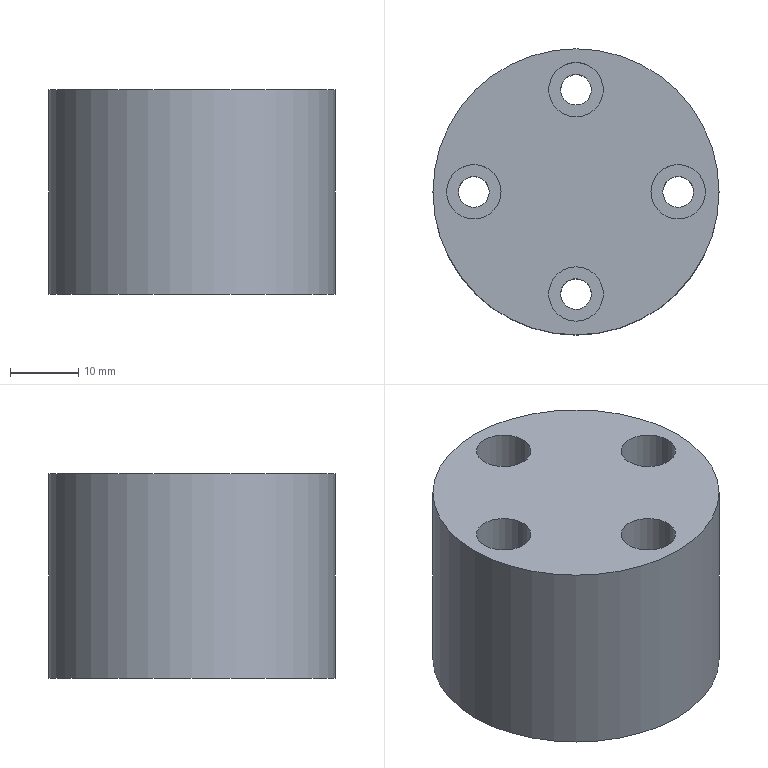Part | NX | 1 solid | 15 faces | box 42 x 42 x 30 mm | volume 38830 mm3 | cylinder 9 | plane 6 | commonest cylinder face diameters 4.5 x4 8 x4 42 x1
STEP:
#1=CARTESIAN_POINT('',(0.,-17.25,-30.));
#2=VERTEX_POINT('',#1);
#3=CARTESIAN_POINT('',(0.,-15.,-30.));
#4=DIRECTION('',(0.,0.,1.));
#5=DIRECTION('',(0.,-1.,0.));
#6=AXIS2_PLACEMENT_3D('',#3,#4,#5);
#7=CIRCLE('',#6,2.25);
#8=EDGE_CURVE('',#2,#2,#7,.T.);
#9=ORIENTED_EDGE('',*,*,#8,.F.);
#10=EDGE_LOOP('',(#9));
#11=FACE_BOUND('',#10,.T.);
#12=CARTESIAN_POINT('',(2.25,-15.,-6.));
#13=VERTEX_POINT('',#12);
#14=CARTESIAN_POINT('',(0.,-15.,-6.));
#15=DIRECTION('',(0.,0.,1.));
#16=DIRECTION('',(1.,0.,0.));
#17=AXIS2_PLACEMENT_3D('',#14,#15,#16);
#18=CIRCLE('',#17,2.25);
#19=EDGE_CURVE('',#13,#13,#18,.T.);
#20=ORIENTED_EDGE('',*,*,#19,.T.);
#21=EDGE_LOOP('',(#20));
#22=FACE_BOUND('',#21,.T.);
#23=CARTESIAN_POINT('',(0.,-15.,0.));
#24=DIRECTION('',(0.,0.,-1.));
#25=DIRECTION('',(-1.,0.,0.));
#26=AXIS2_PLACEMENT_3D('',#23,#24,#25);
#27=CYLINDRICAL_SURFACE('',#26,2.25);
#28=ADVANCED_FACE('',(#11,#22),#27,.F.);
#29=CARTESIAN_POINT('',(0.,17.25,-30.));
#30=VERTEX_POINT('',#29);
#31=CARTESIAN_POINT('',(0.,15.,-30.));
#32=DIRECTION('',(0.,0.,1.));
#33=DIRECTION('',(0.,1.,0.));
#34=AXIS2_PLACEMENT_3D('',#31,#32,#33);
#35=CIRCLE('',#34,2.25);
#36=EDGE_CURVE('',#30,#30,#35,.T.);
#37=ORIENTED_EDGE('',*,*,#36,.F.);
#38=EDGE_LOOP('',(#37));
#39=FACE_BOUND('',#38,.T.);
#40=CARTESIAN_POINT('',(2.25,15.,-6.));
#41=VERTEX_POINT('',#40);
#42=CARTESIAN_POINT('',(0.,15.,-6.));
#43=DIRECTION('',(0.,0.,1.));
#44=DIRECTION('',(1.,0.,0.));
#45=AXIS2_PLACEMENT_3D('',#42,#43,#44);
#46=CIRCLE('',#45,2.25);
#47=EDGE_CURVE('',#41,#41,#46,.T.);
#48=ORIENTED_EDGE('',*,*,#47,.T.);
#49=EDGE_LOOP('',(#48));
#50=FACE_BOUND('',#49,.T.);
#51=CARTESIAN_POINT('',(0.,15.,0.));
#52=DIRECTION('',(0.,0.,-1.));
#53=DIRECTION('',(-1.,0.,0.));
#54=AXIS2_PLACEMENT_3D('',#51,#52,#53);
#55=CYLINDRICAL_SURFACE('',#54,2.25);
#56=ADVANCED_FACE('',(#39,#50),#55,.F.);
#57=CARTESIAN_POINT('',(17.25,0.,-30.));
#58=VERTEX_POINT('',#57);
#59=CARTESIAN_POINT('',(15.,0.,-30.));
#60=DIRECTION('',(0.,0.,1.));
#61=DIRECTION('',(1.,0.,0.));
#62=AXIS2_PLACEMENT_3D('',#59,#60,#61);
#63=CIRCLE('',#62,2.25);
#64=EDGE_CURVE('',#58,#58,#63,.T.);
#65=ORIENTED_EDGE('',*,*,#64,.F.);
#66=EDGE_LOOP('',(#65));
#67=FACE_BOUND('',#66,.T.);
#68=CARTESIAN_POINT('',(17.25,0.,-6.));
#69=VERTEX_POINT('',#68);
#70=CARTESIAN_POINT('',(15.,0.,-6.));
#71=DIRECTION('',(0.,0.,1.));
#72=DIRECTION('',(1.,0.,0.));
#73=AXIS2_PLACEMENT_3D('',#70,#71,#72);
#74=CIRCLE('',#73,2.25);
#75=EDGE_CURVE('',#69,#69,#74,.T.);
#76=ORIENTED_EDGE('',*,*,#75,.T.);
#77=EDGE_LOOP('',(#76));
#78=FACE_BOUND('',#77,.T.);
#79=CARTESIAN_POINT('',(15.,0.,0.));
#80=DIRECTION('',(0.,0.,-1.));
#81=DIRECTION('',(-1.,0.,0.));
#82=AXIS2_PLACEMENT_3D('',#79,#80,#81);
#83=CYLINDRICAL_SURFACE('',#82,2.25);
#84=ADVANCED_FACE('',(#67,#78),#83,.F.);
#85=CARTESIAN_POINT('',(0.,19.,0.));
#86=VERTEX_POINT('',#85);
#87=CARTESIAN_POINT('',(0.,15.,0.));
#88=DIRECTION('',(0.,0.,1.));
#89=DIRECTION('',(0.,1.,0.));
#90=AXIS2_PLACEMENT_3D('',#87,#88,#89);
#91=CIRCLE('',#90,4.);
#92=EDGE_CURVE('',#86,#86,#91,.T.);
#93=ORIENTED_EDGE('',*,*,#92,.F.);
#94=EDGE_LOOP('',(#93));
#95=FACE_BOUND('',#94,.T.);
#96=CARTESIAN_POINT('',(21.,0.,0.));
#97=VERTEX_POINT('',#96);
#98=CARTESIAN_POINT('',(0.,0.,0.));
#99=DIRECTION('',(0.,0.,-1.));
#100=DIRECTION('',(1.,0.,0.));
#101=AXIS2_PLACEMENT_3D('',#98,#99,#100);
#102=CIRCLE('',#101,21.);
#103=EDGE_CURVE('',#97,#97,#102,.T.);
#104=ORIENTED_EDGE('',*,*,#103,.F.);
#105=EDGE_LOOP('',(#104));
#106=FACE_BOUND('',#105,.T.);
#107=CARTESIAN_POINT('',(-19.,0.,0.));
#108=VERTEX_POINT('',#107);
#109=CARTESIAN_POINT('',(-15.,0.,0.));
#110=DIRECTION('',(0.,0.,-1.));
#111=DIRECTION('',(-1.,0.,0.));
#112=AXIS2_PLACEMENT_3D('',#109,#110,#111);
#113=CIRCLE('',#112,4.);
#114=EDGE_CURVE('',#108,#108,#113,.T.);
#115=ORIENTED_EDGE('',*,*,#114,.T.);
#116=EDGE_LOOP('',(#115));
#117=FACE_BOUND('',#116,.T.);
#118=CARTESIAN_POINT('',(0.,-19.,0.));
#119=VERTEX_POINT('',#118);
#120=CARTESIAN_POINT('',(0.,-15.,0.));
#121=DIRECTION('',(0.,0.,1.));
#122=DIRECTION('',(0.,-1.,0.));
#123=AXIS2_PLACEMENT_3D('',#120,#121,#122);
#124=CIRCLE('',#123,4.);
#125=EDGE_CURVE('',#119,#119,#124,.T.);
#126=ORIENTED_EDGE('',*,*,#125,.F.);
#127=EDGE_LOOP('',(#126));
#128=FACE_BOUND('',#127,.T.);
#129=CARTESIAN_POINT('',(19.,0.,0.));
#130=VERTEX_POINT('',#129);
#131=CARTESIAN_POINT('',(15.,0.,0.));
#132=DIRECTION('',(0.,0.,1.));
#133=DIRECTION('',(1.,0.,0.));
#134=AXIS2_PLACEMENT_3D('',#131,#132,#133);
#135=CIRCLE('',#134,4.);
#136=EDGE_CURVE('',#130,#130,#135,.T.);
#137=ORIENTED_EDGE('',*,*,#136,.F.);
#138=EDGE_LOOP('',(#137));
#139=FACE_BOUND('',#138,.T.);
#140=CARTESIAN_POINT('',(7.5,0.,0.));
#141=DIRECTION('',(0.,0.,-1.));
#142=DIRECTION('',(-1.,0.,0.));
#143=AXIS2_PLACEMENT_3D('',#140,#141,#142);
#144=PLANE('',#143);
#145=ADVANCED_FACE('',(#95,#106,#117,#128,#139),#144,.F.);
#146=ORIENTED_EDGE('',*,*,#103,.T.);
#147=EDGE_LOOP('',(#146));
#148=FACE_BOUND('',#147,.T.);
#149=CARTESIAN_POINT('',(21.,0.,-30.));
#150=VERTEX_POINT('',#149);
#151=CARTESIAN_POINT('',(0.,0.,-30.));
#152=DIRECTION('',(0.,0.,-1.));
#153=DIRECTION('',(1.,0.,0.));
#154=AXIS2_PLACEMENT_3D('',#151,#152,#153);
#155=CIRCLE('',#154,21.);
#156=EDGE_CURVE('',#150,#150,#155,.T.);
#157=ORIENTED_EDGE('',*,*,#156,.F.);
#158=EDGE_LOOP('',(#157));
#159=FACE_BOUND('',#158,.T.);
#160=CARTESIAN_POINT('',(0.,0.,0.));
#161=DIRECTION('',(0.,0.,-1.));
#162=DIRECTION('',(-1.,0.,0.));
#163=AXIS2_PLACEMENT_3D('',#160,#161,#162);
#164=CYLINDRICAL_SURFACE('',#163,21.);
#165=ADVANCED_FACE('',(#148,#159),#164,.T.);
#166=CARTESIAN_POINT('',(-17.25,0.,-6.));
#167=VERTEX_POINT('',#166);
#168=CARTESIAN_POINT('',(-15.,0.,-6.));
#169=DIRECTION('',(0.,0.,-1.));
#170=DIRECTION('',(-1.,0.,0.));
#171=AXIS2_PLACEMENT_3D('',#168,#169,#170);
#172=CIRCLE('',#171,2.25);
#173=EDGE_CURVE('',#167,#167,#172,.T.);
#174=ORIENTED_EDGE('',*,*,#173,.F.);
#175=EDGE_LOOP('',(#174));
#176=FACE_BOUND('',#175,.T.);
#177=CARTESIAN_POINT('',(-17.25,0.,-30.));
#178=VERTEX_POINT('',#177);
#179=CARTESIAN_POINT('',(-15.,0.,-30.));
#180=DIRECTION('',(0.,0.,1.));
#181=DIRECTION('',(-1.,0.,0.));
#182=AXIS2_PLACEMENT_3D('',#179,#180,#181);
#183=CIRCLE('',#182,2.25);
#184=EDGE_CURVE('',#178,#178,#183,.T.);
#185=ORIENTED_EDGE('',*,*,#184,.F.);
#186=EDGE_LOOP('',(#185));
#187=FACE_BOUND('',#186,.T.);
#188=CARTESIAN_POINT('',(-15.,0.,0.));
#189=DIRECTION('',(0.,0.,-1.));
#190=DIRECTION('',(-1.,0.,0.));
#191=AXIS2_PLACEMENT_3D('',#188,#189,#190);
#192=CYLINDRICAL_SURFACE('',#191,2.25);
#193=ADVANCED_FACE('',(#176,#187),#192,.F.);
#194=ORIENTED_EDGE('',*,*,#156,.T.);
#195=EDGE_LOOP('',(#194));
#196=FACE_BOUND('',#195,.T.);
#197=ORIENTED_EDGE('',*,*,#64,.T.);
#198=EDGE_LOOP('',(#197));
#199=FACE_BOUND('',#198,.T.);
#200=ORIENTED_EDGE('',*,*,#36,.T.);
#201=EDGE_LOOP('',(#200));
#202=FACE_BOUND('',#201,.T.);
#203=ORIENTED_EDGE('',*,*,#8,.T.);
#204=EDGE_LOOP('',(#203));
#205=FACE_BOUND('',#204,.T.);
#206=ORIENTED_EDGE('',*,*,#184,.T.);
#207=EDGE_LOOP('',(#206));
#208=FACE_BOUND('',#207,.T.);
#209=CARTESIAN_POINT('',(7.5,0.,-30.));
#210=DIRECTION('',(0.,0.,-1.));
#211=DIRECTION('',(-1.,0.,0.));
#212=AXIS2_PLACEMENT_3D('',#209,#210,#211);
#213=PLANE('',#212);
#214=ADVANCED_FACE('',(#196,#199,#202,#205,#208),#213,.T.);
#215=ORIENTED_EDGE('',*,*,#114,.F.);
#216=EDGE_LOOP('',(#215));
#217=FACE_BOUND('',#216,.T.);
#218=CARTESIAN_POINT('',(-19.,0.,-6.));
#219=VERTEX_POINT('',#218);
#220=CARTESIAN_POINT('',(-15.,0.,-6.));
#221=DIRECTION('',(0.,0.,-1.));
#222=DIRECTION('',(-1.,0.,0.));
#223=AXIS2_PLACEMENT_3D('',#220,#221,#222);
#224=CIRCLE('',#223,4.);
#225=EDGE_CURVE('',#219,#219,#224,.F.);
#226=ORIENTED_EDGE('',*,*,#225,.F.);
#227=EDGE_LOOP('',(#226));
#228=FACE_BOUND('',#227,.T.);
#229=CARTESIAN_POINT('',(-15.,0.,0.));
#230=DIRECTION('',(0.,0.,-1.));
#231=DIRECTION('',(-1.,0.,0.));
#232=AXIS2_PLACEMENT_3D('',#229,#230,#231);
#233=CYLINDRICAL_SURFACE('',#232,4.);
#234=ADVANCED_FACE('',(#217,#228),#233,.F.);
#235=ORIENTED_EDGE('',*,*,#173,.T.);
#236=EDGE_LOOP('',(#235));
#237=FACE_BOUND('',#236,.T.);
#238=ORIENTED_EDGE('',*,*,#225,.T.);
#239=EDGE_LOOP('',(#238));
#240=FACE_BOUND('',#239,.T.);
#241=CARTESIAN_POINT('',(-15.,0.,-6.));
#242=DIRECTION('',(0.,0.,-1.));
#243=DIRECTION('',(-1.,0.,0.));
#244=AXIS2_PLACEMENT_3D('',#241,#242,#243);
#245=PLANE('',#244);
#246=ADVANCED_FACE('',(#237,#240),#245,.F.);
#247=ORIENTED_EDGE('',*,*,#125,.T.);
#248=EDGE_LOOP('',(#247));
#249=FACE_BOUND('',#248,.T.);
#250=CARTESIAN_POINT('',(0.,-19.,-6.));
#251=VERTEX_POINT('',#250);
#252=CARTESIAN_POINT('',(0.,-15.,-6.));
#253=DIRECTION('',(0.,0.,1.));
#254=DIRECTION('',(0.,-1.,0.));
#255=AXIS2_PLACEMENT_3D('',#252,#253,#254);
#256=CIRCLE('',#255,4.);
#257=EDGE_CURVE('',#251,#251,#256,.F.);
#258=ORIENTED_EDGE('',*,*,#257,.T.);
#259=EDGE_LOOP('',(#258));
#260=FACE_BOUND('',#259,.T.);
#261=CARTESIAN_POINT('',(0.,-15.,0.));
#262=DIRECTION('',(0.,0.,-1.));
#263=DIRECTION('',(-1.,0.,0.));
#264=AXIS2_PLACEMENT_3D('',#261,#262,#263);
#265=CYLINDRICAL_SURFACE('',#264,4.);
#266=ADVANCED_FACE('',(#249,#260),#265,.F.);
#267=ORIENTED_EDGE('',*,*,#19,.F.);
#268=EDGE_LOOP('',(#267));
#269=FACE_BOUND('',#268,.T.);
#270=ORIENTED_EDGE('',*,*,#257,.F.);
#271=EDGE_LOOP('',(#270));
#272=FACE_BOUND('',#271,.T.);
#273=CARTESIAN_POINT('',(0.,-15.,-6.));
#274=DIRECTION('',(0.,0.,1.));
#275=DIRECTION('',(1.,0.,0.));
#276=AXIS2_PLACEMENT_3D('',#273,#274,#275);
#277=PLANE('',#276);
#278=ADVANCED_FACE('',(#269,#272),#277,.T.);
#279=ORIENTED_EDGE('',*,*,#92,.T.);
#280=EDGE_LOOP('',(#279));
#281=FACE_BOUND('',#280,.T.);
#282=CARTESIAN_POINT('',(0.,19.,-6.));
#283=VERTEX_POINT('',#282);
#284=CARTESIAN_POINT('',(0.,15.,-6.));
#285=DIRECTION('',(0.,0.,1.));
#286=DIRECTION('',(0.,1.,0.));
#287=AXIS2_PLACEMENT_3D('',#284,#285,#286);
#288=CIRCLE('',#287,4.);
#289=EDGE_CURVE('',#283,#283,#288,.F.);
#290=ORIENTED_EDGE('',*,*,#289,.T.);
#291=EDGE_LOOP('',(#290));
#292=FACE_BOUND('',#291,.T.);
#293=CARTESIAN_POINT('',(0.,15.,0.));
#294=DIRECTION('',(0.,0.,-1.));
#295=DIRECTION('',(-1.,0.,0.));
#296=AXIS2_PLACEMENT_3D('',#293,#294,#295);
#297=CYLINDRICAL_SURFACE('',#296,4.);
#298=ADVANCED_FACE('',(#281,#292),#297,.F.);
#299=ORIENTED_EDGE('',*,*,#47,.F.);
#300=EDGE_LOOP('',(#299));
#301=FACE_BOUND('',#300,.T.);
#302=ORIENTED_EDGE('',*,*,#289,.F.);
#303=EDGE_LOOP('',(#302));
#304=FACE_BOUND('',#303,.T.);
#305=CARTESIAN_POINT('',(0.,15.,-6.));
#306=DIRECTION('',(0.,0.,1.));
#307=DIRECTION('',(1.,0.,0.));
#308=AXIS2_PLACEMENT_3D('',#305,#306,#307);
#309=PLANE('',#308);
#310=ADVANCED_FACE('',(#301,#304),#309,.T.);
#311=ORIENTED_EDGE('',*,*,#136,.T.);
#312=EDGE_LOOP('',(#311));
#313=FACE_BOUND('',#312,.T.);
#314=CARTESIAN_POINT('',(19.,0.,-6.));
#315=VERTEX_POINT('',#314);
#316=CARTESIAN_POINT('',(15.,0.,-6.));
#317=DIRECTION('',(0.,0.,1.));
#318=DIRECTION('',(1.,0.,0.));
#319=AXIS2_PLACEMENT_3D('',#316,#317,#318);
#320=CIRCLE('',#319,4.);
#321=EDGE_CURVE('',#315,#315,#320,.F.);
#322=ORIENTED_EDGE('',*,*,#321,.T.);
#323=EDGE_LOOP('',(#322));
#324=FACE_BOUND('',#323,.T.);
#325=CARTESIAN_POINT('',(15.,0.,0.));
#326=DIRECTION('',(0.,0.,-1.));
#327=DIRECTION('',(-1.,0.,0.));
#328=AXIS2_PLACEMENT_3D('',#325,#326,#327);
#329=CYLINDRICAL_SURFACE('',#328,4.);
#330=ADVANCED_FACE('',(#313,#324),#329,.F.);
#331=ORIENTED_EDGE('',*,*,#75,.F.);
#332=EDGE_LOOP('',(#331));
#333=FACE_BOUND('',#332,.T.);
#334=ORIENTED_EDGE('',*,*,#321,.F.);
#335=EDGE_LOOP('',(#334));
#336=FACE_BOUND('',#335,.T.);
#337=CARTESIAN_POINT('',(15.,0.,-6.));
#338=DIRECTION('',(0.,0.,1.));
#339=DIRECTION('',(1.,0.,0.));
#340=AXIS2_PLACEMENT_3D('',#337,#338,#339);
#341=PLANE('',#340);
#342=ADVANCED_FACE('',(#333,#336),#341,.T.);
#343=CLOSED_SHELL('',(#28,#56,#84,#145,#165,#193,#214,#234,#246,#266,#278,#298,#310,#330,#342));
#344=MANIFOLD_SOLID_BREP('',#343);
#345=(LENGTH_UNIT()NAMED_UNIT(*)SI_UNIT(.MILLI.,.METRE.));
#346=UNCERTAINTY_MEASURE_WITH_UNIT(LENGTH_MEASURE(0.00001),#345,'','');
#347=(NAMED_UNIT(*)PLANE_ANGLE_UNIT()SI_UNIT($,.RADIAN.));
#348=(NAMED_UNIT(*)SI_UNIT($,.STERADIAN.)SOLID_ANGLE_UNIT());
#349=(GEOMETRIC_REPRESENTATION_CONTEXT(3)GLOBAL_UNCERTAINTY_ASSIGNED_CONTEXT((#346))GLOBAL_UNIT_ASSIGNED_CONTEXT((#345,#347,#348))REPRESENTATION_CONTEXT('',''));
#350=ADVANCED_BREP_SHAPE_REPRESENTATION('',(#344),#349);